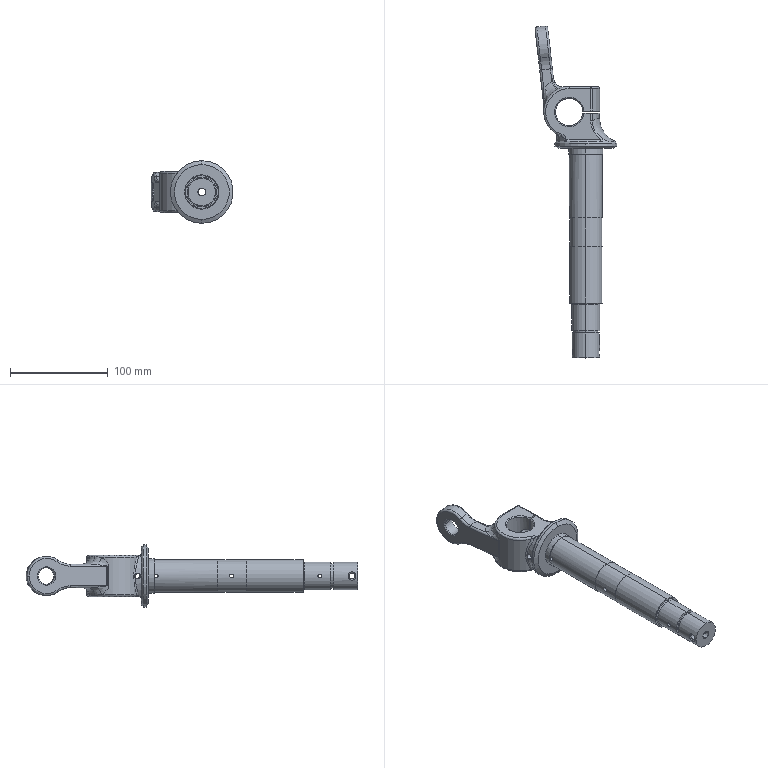Part | SolidWorks | features HoleWzd 10, 3DProfileFeature 3, Fillet 3, Chamfer 2, ICE 2, BaseBody 1, RevCut 1 | 1 solid | 168 faces | box 83.814 x 338.849 x 64 mm | volume 286212 mm3 | cylinder 88 | spline 26 | plane 25 | torus 14 | cone 13 | sphere 2 | commonest cylinder face diameters 4 x26 6 x10 12 x6 12.5 x5 5 x4 33.5 x4